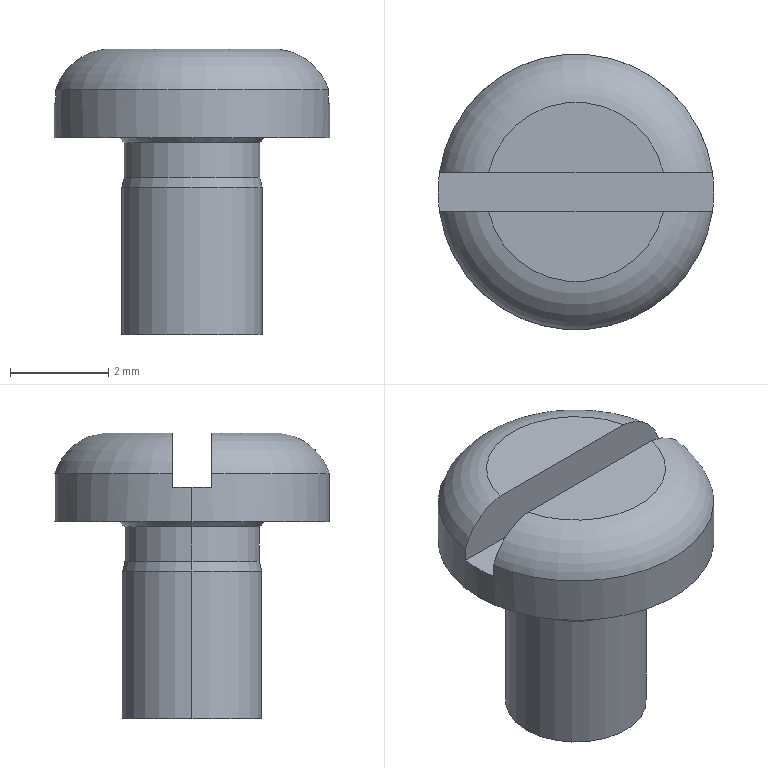Part | SolidWorks | features ICE 3, Revolution 2, Extrusion 1, RevCut 1 | 1 solid | 19 faces | box 5.6 x 5.6 x 5.8 mm | volume 61.126 mm3 | plane 7 | cylinder 6 | torus 4 | cone 2 | commonest cylinder face diameters 2.75 x2 2.85 x2 5.6 x2
STEP:
#1=CARTESIAN_POINT('',(-1.425,0.,-4.));
#2=VERTEX_POINT('',#1);
#3=CARTESIAN_POINT('',(1.425,0.,-4.));
#4=VERTEX_POINT('',#3);
#5=CARTESIAN_POINT('',(0.,0.,-4.));
#6=DIRECTION('',(0.,0.,-1.));
#7=DIRECTION('',(-1.,0.,0.));
#8=AXIS2_PLACEMENT_3D('',#5,#6,#7);
#9=CIRCLE('',#8,1.425);
#10=EDGE_CURVE('',#2,#4,#9,.T.);
#11=ORIENTED_EDGE('',*,*,#10,.F.);
#12=CARTESIAN_POINT('',(-1.425,0.,-1.));
#13=VERTEX_POINT('',#12);
#14=CARTESIAN_POINT('',(-1.425,0.,-4.));
#15=DIRECTION('',(0.,0.,1.));
#16=VECTOR('',#15,1000.);
#17=LINE('',#14,#16);
#18=EDGE_CURVE('',#2,#13,#17,.T.);
#19=ORIENTED_EDGE('',*,*,#18,.T.);
#20=CARTESIAN_POINT('',(1.425,0.,-1.));
#21=VERTEX_POINT('',#20);
#22=CARTESIAN_POINT('',(0.,0.,-1.));
#23=DIRECTION('',(0.,0.,-1.));
#24=DIRECTION('',(-1.,0.,0.));
#25=AXIS2_PLACEMENT_3D('',#22,#23,#24);
#26=CIRCLE('',#25,1.425);
#27=EDGE_CURVE('',#13,#21,#26,.T.);
#28=ORIENTED_EDGE('',*,*,#27,.T.);
#29=CARTESIAN_POINT('',(1.425,0.,-4.));
#30=DIRECTION('',(0.,0.,1.));
#31=VECTOR('',#30,1000.);
#32=LINE('',#29,#31);
#33=EDGE_CURVE('',#4,#21,#32,.T.);
#34=ORIENTED_EDGE('',*,*,#33,.F.);
#35=EDGE_LOOP('',(#11,#19,#28,#34));
#36=FACE_OUTER_BOUND('',#35,.T.);
#37=CARTESIAN_POINT('',(0.,0.,-4.));
#38=DIRECTION('',(0.,0.,1.));
#39=DIRECTION('',(1.,0.,0.));
#40=AXIS2_PLACEMENT_3D('',#37,#38,#39);
#41=CYLINDRICAL_SURFACE('',#40,1.425);
#42=ADVANCED_FACE('',(#36),#41,.T.);
#43=CARTESIAN_POINT('',(-1.375,0.,-0.8));
#44=VERTEX_POINT('',#43);
#45=CARTESIAN_POINT('',(1.375,0.,-0.8));
#46=VERTEX_POINT('',#45);
#47=CARTESIAN_POINT('',(0.,0.,-0.8));
#48=DIRECTION('',(0.,0.,-1.));
#49=DIRECTION('',(-1.,0.,0.));
#50=AXIS2_PLACEMENT_3D('',#47,#48,#49);
#51=CIRCLE('',#50,1.375);
#52=EDGE_CURVE('',#44,#46,#51,.T.);
#53=ORIENTED_EDGE('',*,*,#52,.T.);
#54=CARTESIAN_POINT('',(1.375,0.,-0.8));
#55=DIRECTION('',(0.2425,0.,-0.9701));
#56=VECTOR('',#55,1000.);
#57=LINE('',#54,#56);
#58=EDGE_CURVE('',#46,#21,#57,.T.);
#59=ORIENTED_EDGE('',*,*,#58,.T.);
#60=ORIENTED_EDGE('',*,*,#27,.F.);
#61=CARTESIAN_POINT('',(-1.375,0.,-0.8));
#62=DIRECTION('',(-0.2425,0.,-0.9701));
#63=VECTOR('',#62,1000.);
#64=LINE('',#61,#63);
#65=EDGE_CURVE('',#44,#13,#64,.T.);
#66=ORIENTED_EDGE('',*,*,#65,.F.);
#67=EDGE_LOOP('',(#53,#59,#60,#66));
#68=FACE_OUTER_BOUND('',#67,.T.);
#69=CARTESIAN_POINT('',(0.,0.,-0.8));
#70=DIRECTION('',(0.,0.,-1.));
#71=DIRECTION('',(-1.,0.,0.));
#72=AXIS2_PLACEMENT_3D('',#69,#70,#71);
#73=CONICAL_SURFACE('',#72,1.375,0.245);
#74=ADVANCED_FACE('',(#68),#73,.T.);
#75=ORIENTED_EDGE('',*,*,#52,.F.);
#76=CARTESIAN_POINT('',(-1.375,0.,-0.1));
#77=VERTEX_POINT('',#76);
#78=CARTESIAN_POINT('',(-1.375,0.,-0.8));
#79=DIRECTION('',(0.,0.,1.));
#80=VECTOR('',#79,1000.);
#81=LINE('',#78,#80);
#82=EDGE_CURVE('',#44,#77,#81,.T.);
#83=ORIENTED_EDGE('',*,*,#82,.T.);
#84=CARTESIAN_POINT('',(1.375,0.,-0.1));
#85=VERTEX_POINT('',#84);
#86=CARTESIAN_POINT('',(0.,0.,-0.1));
#87=DIRECTION('',(0.,0.,-1.));
#88=DIRECTION('',(-1.,0.,0.));
#89=AXIS2_PLACEMENT_3D('',#86,#87,#88);
#90=CIRCLE('',#89,1.375);
#91=EDGE_CURVE('',#77,#85,#90,.T.);
#92=ORIENTED_EDGE('',*,*,#91,.T.);
#93=CARTESIAN_POINT('',(1.375,0.,-0.8));
#94=DIRECTION('',(0.,0.,1.));
#95=VECTOR('',#94,1000.);
#96=LINE('',#93,#95);
#97=EDGE_CURVE('',#46,#85,#96,.T.);
#98=ORIENTED_EDGE('',*,*,#97,.F.);
#99=EDGE_LOOP('',(#75,#83,#92,#98));
#100=FACE_OUTER_BOUND('',#99,.T.);
#101=CARTESIAN_POINT('',(0.,0.,-0.8));
#102=DIRECTION('',(0.,0.,1.));
#103=DIRECTION('',(1.,0.,0.));
#104=AXIS2_PLACEMENT_3D('',#101,#102,#103);
#105=CYLINDRICAL_SURFACE('',#104,1.375);
#106=ADVANCED_FACE('',(#100),#105,.T.);
#107=CARTESIAN_POINT('',(-1.475,0.,0.));
#108=VERTEX_POINT('',#107);
#109=CARTESIAN_POINT('',(1.475,0.,0.));
#110=VERTEX_POINT('',#109);
#111=CARTESIAN_POINT('',(0.,0.,0.));
#112=DIRECTION('',(0.,0.,1.));
#113=DIRECTION('',(1.,0.,0.));
#114=AXIS2_PLACEMENT_3D('',#111,#112,#113);
#115=CIRCLE('',#114,1.475);
#116=EDGE_CURVE('',#108,#110,#115,.T.);
#117=ORIENTED_EDGE('',*,*,#116,.F.);
#118=CARTESIAN_POINT('',(-2.048,0.,-0.673));
#119=DIRECTION('',(0.,1.,0.));
#120=DIRECTION('',(-1.,0.,0.));
#121=AXIS2_PLACEMENT_3D('',#118,#119,#120);
#122=CIRCLE('',#121,0.8839);
#123=EDGE_CURVE('',#108,#77,#122,.T.);
#124=ORIENTED_EDGE('',*,*,#123,.T.);
#125=CARTESIAN_POINT('',(0.,0.,-0.1));
#126=DIRECTION('',(0.,0.,-1.));
#127=DIRECTION('',(-1.,0.,0.));
#128=AXIS2_PLACEMENT_3D('',#125,#126,#127);
#129=CIRCLE('',#128,1.375);
#130=EDGE_CURVE('',#85,#77,#129,.T.);
#131=ORIENTED_EDGE('',*,*,#130,.F.);
#132=CARTESIAN_POINT('',(2.048,0.,-0.673));
#133=DIRECTION('',(0.,-1.,0.));
#134=DIRECTION('',(0.,0.,-1.));
#135=AXIS2_PLACEMENT_3D('',#132,#133,#134);
#136=CIRCLE('',#135,0.8839);
#137=EDGE_CURVE('',#110,#85,#136,.T.);
#138=ORIENTED_EDGE('',*,*,#137,.F.);
#139=EDGE_LOOP('',(#117,#124,#131,#138));
#140=FACE_OUTER_BOUND('',#139,.T.);
#141=CARTESIAN_POINT('',(0.,0.,-0.673));
#142=DIRECTION('',(0.,0.,1.));
#143=DIRECTION('',(1.,0.,0.));
#144=AXIS2_PLACEMENT_3D('',#141,#142,#143);
#145=TOROIDAL_SURFACE('',#144,2.048,0.8839);
#146=ADVANCED_FACE('',(#140),#145,.F.);
#147=CARTESIAN_POINT('',(2.771,0.4,0.7));
#148=VERTEX_POINT('',#147);
#149=CARTESIAN_POINT('',(2.8,0.,0.7));
#150=VERTEX_POINT('',#149);
#151=CARTESIAN_POINT('',(0.,0.,0.7));
#152=DIRECTION('',(0.,0.,-1.));
#153=DIRECTION('',(-1.,0.,0.));
#154=AXIS2_PLACEMENT_3D('',#151,#152,#153);
#155=CIRCLE('',#154,2.8);
#156=EDGE_CURVE('',#148,#150,#155,.T.);
#157=ORIENTED_EDGE('',*,*,#156,.T.);
#158=CARTESIAN_POINT('',(2.8,0.,0.));
#159=VERTEX_POINT('',#158);
#160=CARTESIAN_POINT('',(2.8,0.,1.8));
#161=DIRECTION('',(0.,0.,-1.));
#162=VECTOR('',#161,1000.);
#163=LINE('',#160,#162);
#164=EDGE_CURVE('',#150,#159,#163,.T.);
#165=ORIENTED_EDGE('',*,*,#164,.T.);
#166=CARTESIAN_POINT('',(-2.8,0.,0.));
#167=VERTEX_POINT('',#166);
#168=CARTESIAN_POINT('',(0.,0.,0.));
#169=DIRECTION('',(0.,0.,1.));
#170=DIRECTION('',(1.,0.,0.));
#171=AXIS2_PLACEMENT_3D('',#168,#169,#170);
#172=CIRCLE('',#171,2.8);
#173=EDGE_CURVE('',#159,#167,#172,.T.);
#174=ORIENTED_EDGE('',*,*,#173,.T.);
#175=CARTESIAN_POINT('',(-2.8,0.,0.7));
#176=VERTEX_POINT('',#175);
#177=CARTESIAN_POINT('',(-2.8,0.,1.8));
#178=DIRECTION('',(0.,0.,-1.));
#179=VECTOR('',#178,1000.);
#180=LINE('',#177,#179);
#181=EDGE_CURVE('',#176,#167,#180,.T.);
#182=ORIENTED_EDGE('',*,*,#181,.F.);
#183=CARTESIAN_POINT('',(-2.771,0.4,0.7));
#184=VERTEX_POINT('',#183);
#185=CARTESIAN_POINT('',(0.,0.,0.7));
#186=DIRECTION('',(0.,0.,-1.));
#187=DIRECTION('',(-1.,0.,0.));
#188=AXIS2_PLACEMENT_3D('',#185,#186,#187);
#189=CIRCLE('',#188,2.8);
#190=EDGE_CURVE('',#176,#184,#189,.T.);
#191=ORIENTED_EDGE('',*,*,#190,.T.);
#192=CARTESIAN_POINT('',(-2.771,0.4,0.98));
#193=VERTEX_POINT('',#192);
#194=CARTESIAN_POINT('',(-2.771,0.4,1.8));
#195=DIRECTION('',(0.,0.,1.));
#196=VECTOR('',#195,1000.);
#197=LINE('',#194,#196);
#198=EDGE_CURVE('',#184,#193,#197,.T.);
#199=ORIENTED_EDGE('',*,*,#198,.T.);
#200=CARTESIAN_POINT('',(2.771,0.4,0.98));
#201=VERTEX_POINT('',#200);
#202=CARTESIAN_POINT('',(0.,0.,0.98));
#203=DIRECTION('',(0.,0.,-1.));
#204=DIRECTION('',(-1.,0.,0.));
#205=AXIS2_PLACEMENT_3D('',#202,#203,#204);
#206=CIRCLE('',#205,2.8);
#207=EDGE_CURVE('',#193,#201,#206,.T.);
#208=ORIENTED_EDGE('',*,*,#207,.T.);
#209=CARTESIAN_POINT('',(2.771,0.4,1.8));
#210=DIRECTION('',(0.,0.,-1.));
#211=VECTOR('',#210,1000.);
#212=LINE('',#209,#211);
#213=EDGE_CURVE('',#201,#148,#212,.T.);
#214=ORIENTED_EDGE('',*,*,#213,.T.);
#215=EDGE_LOOP('',(#157,#165,#174,#182,#191,#199,#208,#214));
#216=FACE_OUTER_BOUND('',#215,.T.);
#217=CARTESIAN_POINT('',(0.,0.,1.8));
#218=DIRECTION('',(0.,0.,-1.));
#219=DIRECTION('',(-1.,0.,0.));
#220=AXIS2_PLACEMENT_3D('',#217,#218,#219);
#221=CYLINDRICAL_SURFACE('',#220,2.8);
#222=ADVANCED_FACE('',(#216),#221,.T.);
#223=CARTESIAN_POINT('',(-2.771,-0.4,0.98));
#224=VERTEX_POINT('',#223);
#225=CARTESIAN_POINT('',(-1.775,-0.4,1.8));
#226=VERTEX_POINT('',#225);
#227=CARTESIAN_POINT('',(-2.771,-0.4,0.98));
#228=CARTESIAN_POINT('',(-2.737,-0.4,1.088));
#229=CARTESIAN_POINT('',(-2.687,-0.4,1.191));
#230=CARTESIAN_POINT('',(-2.559,-0.4,1.38));
#231=CARTESIAN_POINT('',(-2.481,-0.4,1.465));
#232=CARTESIAN_POINT('',(-2.306,-0.4,1.608));
#233=CARTESIAN_POINT('',(-2.207,-0.4,1.667));
#234=CARTESIAN_POINT('',(-1.998,-0.4,1.756));
#235=CARTESIAN_POINT('',(-1.889,-0.4,1.786));
#236=CARTESIAN_POINT('',(-1.775,-0.4,1.8));
#237=B_SPLINE_CURVE_WITH_KNOTS('',3,(#227,#228,#229,#230,#231,#232,#233,#234,#235,#236),.UNSPECIFIED.,.F.,.F.,(4,2,2,2,4),(0.00711,0.007449,0.007788,0.008126,0.008465),.UNSPECIFIED.);
#238=EDGE_CURVE('',#224,#226,#237,.T.);
#239=ORIENTED_EDGE('',*,*,#238,.F.);
#240=CARTESIAN_POINT('',(2.771,-0.4,0.98));
#241=VERTEX_POINT('',#240);
#242=CARTESIAN_POINT('',(0.,0.,0.98));
#243=DIRECTION('',(0.,0.,-1.));
#244=DIRECTION('',(-1.,0.,0.));
#245=AXIS2_PLACEMENT_3D('',#242,#243,#244);
#246=CIRCLE('',#245,2.8);
#247=EDGE_CURVE('',#241,#224,#246,.T.);
#248=ORIENTED_EDGE('',*,*,#247,.F.);
#249=CARTESIAN_POINT('',(1.775,-0.4,1.8));
#250=VERTEX_POINT('',#249);
#251=CARTESIAN_POINT('',(1.775,-0.4,1.8));
#252=CARTESIAN_POINT('',(2.,-0.4,1.772));
#253=CARTESIAN_POINT('',(2.219,-0.4,1.679));
#254=CARTESIAN_POINT('',(2.482,-0.4,1.464));
#255=CARTESIAN_POINT('',(2.559,-0.4,1.379));
#256=CARTESIAN_POINT('',(2.687,-0.4,1.191));
#257=CARTESIAN_POINT('',(2.737,-0.4,1.089));
#258=CARTESIAN_POINT('',(2.771,-0.4,0.98));
#259=B_SPLINE_CURVE_WITH_KNOTS('',3,(#251,#252,#253,#254,#255,#256,#257,#258),.UNSPECIFIED.,.F.,.F.,(4,2,2,4),(0.001738,0.002418,0.002758,0.003097),.UNSPECIFIED.);
#260=EDGE_CURVE('',#250,#241,#259,.T.);
#261=ORIENTED_EDGE('',*,*,#260,.F.);
#262=CARTESIAN_POINT('',(0.,0.,1.8));
#263=DIRECTION('',(0.,0.,-1.));
#264=DIRECTION('',(-1.,0.,0.));
#265=AXIS2_PLACEMENT_3D('',#262,#263,#264);
#266=CIRCLE('',#265,1.82);
#267=EDGE_CURVE('',#250,#226,#266,.T.);
#268=ORIENTED_EDGE('',*,*,#267,.T.);
#269=EDGE_LOOP('',(#239,#248,#261,#268));
#270=FACE_OUTER_BOUND('',#269,.T.);
#271=CARTESIAN_POINT('',(0.,0.,0.624));
#272=DIRECTION('',(0.,0.,-1.));
#273=DIRECTION('',(-1.,0.,0.));
#274=AXIS2_PLACEMENT_3D('',#271,#272,#273);
#275=TOROIDAL_SURFACE('',#274,1.669,1.186);
#276=ADVANCED_FACE('',(#270),#275,.T.);
#277=CARTESIAN_POINT('',(0.,-0.4,1.8));
#278=DIRECTION('',(1.,0.,0.));
#279=VECTOR('',#278,1000.);
#280=LINE('',#277,#279);
#281=EDGE_CURVE('',#226,#250,#280,.T.);
#282=ORIENTED_EDGE('',*,*,#281,.F.);
#283=ORIENTED_EDGE('',*,*,#267,.F.);
#284=EDGE_LOOP('',(#282,#283));
#285=FACE_OUTER_BOUND('',#284,.T.);
#286=CARTESIAN_POINT('',(0.,0.,1.8));
#287=DIRECTION('',(0.,0.,1.));
#288=DIRECTION('',(1.,0.,0.));
#289=AXIS2_PLACEMENT_3D('',#286,#287,#288);
#290=PLANE('',#289);
#291=ADVANCED_FACE('',(#285),#290,.T.);
#292=ORIENTED_EDGE('',*,*,#164,.F.);
#293=CARTESIAN_POINT('',(2.771,-0.4,0.7));
#294=VERTEX_POINT('',#293);
#295=CARTESIAN_POINT('',(0.,0.,0.7));
#296=DIRECTION('',(0.,0.,-1.));
#297=DIRECTION('',(-1.,0.,0.));
#298=AXIS2_PLACEMENT_3D('',#295,#296,#297);
#299=CIRCLE('',#298,2.8);
#300=EDGE_CURVE('',#150,#294,#299,.T.);
#301=ORIENTED_EDGE('',*,*,#300,.T.);
#302=CARTESIAN_POINT('',(2.771,-0.4,1.8));
#303=DIRECTION('',(0.,0.,1.));
#304=VECTOR('',#303,1000.);
#305=LINE('',#302,#304);
#306=EDGE_CURVE('',#294,#241,#305,.T.);
#307=ORIENTED_EDGE('',*,*,#306,.T.);
#308=ORIENTED_EDGE('',*,*,#247,.T.);
#309=CARTESIAN_POINT('',(-2.771,-0.4,0.7));
#310=VERTEX_POINT('',#309);
#311=CARTESIAN_POINT('',(-2.771,-0.4,1.8));
#312=DIRECTION('',(0.,0.,-1.));
#313=VECTOR('',#312,1000.);
#314=LINE('',#311,#313);
#315=EDGE_CURVE('',#224,#310,#314,.T.);
#316=ORIENTED_EDGE('',*,*,#315,.T.);
#317=CARTESIAN_POINT('',(0.,0.,0.7));
#318=DIRECTION('',(0.,0.,-1.));
#319=DIRECTION('',(-1.,0.,0.));
#320=AXIS2_PLACEMENT_3D('',#317,#318,#319);
#321=CIRCLE('',#320,2.8);
#322=EDGE_CURVE('',#310,#176,#321,.T.);
#323=ORIENTED_EDGE('',*,*,#322,.T.);
#324=ORIENTED_EDGE('',*,*,#181,.T.);
#325=CARTESIAN_POINT('',(0.,0.,0.));
#326=DIRECTION('',(0.,0.,1.));
#327=DIRECTION('',(1.,0.,0.));
#328=AXIS2_PLACEMENT_3D('',#325,#326,#327);
#329=CIRCLE('',#328,2.8);
#330=EDGE_CURVE('',#167,#159,#329,.T.);
#331=ORIENTED_EDGE('',*,*,#330,.T.);
#332=EDGE_LOOP('',(#292,#301,#307,#308,#316,#323,#324,#331));
#333=FACE_OUTER_BOUND('',#332,.T.);
#334=CARTESIAN_POINT('',(0.,0.,1.8));
#335=DIRECTION('',(0.,0.,-1.));
#336=DIRECTION('',(-1.,0.,0.));
#337=AXIS2_PLACEMENT_3D('',#334,#335,#336);
#338=CYLINDRICAL_SURFACE('',#337,2.8);
#339=ADVANCED_FACE('',(#333),#338,.T.);
#340=CARTESIAN_POINT('',(0.,0.,0.));
#341=DIRECTION('',(0.,0.,1.));
#342=DIRECTION('',(1.,0.,0.));
#343=AXIS2_PLACEMENT_3D('',#340,#341,#342);
#344=CIRCLE('',#343,1.475);
#345=EDGE_CURVE('',#110,#108,#344,.T.);
#346=ORIENTED_EDGE('',*,*,#345,.T.);
#347=ORIENTED_EDGE('',*,*,#116,.T.);
#348=EDGE_LOOP('',(#346,#347));
#349=FACE_BOUND('',#348,.T.);
#350=ORIENTED_EDGE('',*,*,#330,.F.);
#351=ORIENTED_EDGE('',*,*,#173,.F.);
#352=EDGE_LOOP('',(#350,#351));
#353=FACE_OUTER_BOUND('',#352,.T.);
#354=CARTESIAN_POINT('',(0.,0.,0.));
#355=DIRECTION('',(0.,0.,1.));
#356=DIRECTION('',(1.,0.,0.));
#357=AXIS2_PLACEMENT_3D('',#354,#355,#356);
#358=PLANE('',#357);
#359=ADVANCED_FACE('',(#349,#353),#358,.F.);
#360=ORIENTED_EDGE('',*,*,#123,.F.);
#361=ORIENTED_EDGE('',*,*,#345,.F.);
#362=ORIENTED_EDGE('',*,*,#137,.T.);
#363=ORIENTED_EDGE('',*,*,#91,.F.);
#364=EDGE_LOOP('',(#360,#361,#362,#363));
#365=FACE_OUTER_BOUND('',#364,.T.);
#366=CARTESIAN_POINT('',(0.,0.,-0.673));
#367=DIRECTION('',(0.,0.,1.));
#368=DIRECTION('',(1.,0.,0.));
#369=AXIS2_PLACEMENT_3D('',#366,#367,#368);
#370=TOROIDAL_SURFACE('',#369,2.048,0.8839);
#371=ADVANCED_FACE('',(#365),#370,.F.);
#372=ORIENTED_EDGE('',*,*,#82,.F.);
#373=CARTESIAN_POINT('',(0.,0.,-0.8));
#374=DIRECTION('',(0.,0.,-1.));
#375=DIRECTION('',(-1.,0.,0.));
#376=AXIS2_PLACEMENT_3D('',#373,#374,#375);
#377=CIRCLE('',#376,1.375);
#378=EDGE_CURVE('',#46,#44,#377,.T.);
#379=ORIENTED_EDGE('',*,*,#378,.F.);
#380=ORIENTED_EDGE('',*,*,#97,.T.);
#381=ORIENTED_EDGE('',*,*,#130,.T.);
#382=EDGE_LOOP('',(#372,#379,#380,#381));
#383=FACE_OUTER_BOUND('',#382,.T.);
#384=CARTESIAN_POINT('',(0.,0.,-0.8));
#385=DIRECTION('',(0.,0.,1.));
#386=DIRECTION('',(1.,0.,0.));
#387=AXIS2_PLACEMENT_3D('',#384,#385,#386);
#388=CYLINDRICAL_SURFACE('',#387,1.375);
#389=ADVANCED_FACE('',(#383),#388,.T.);
#390=ORIENTED_EDGE('',*,*,#58,.F.);
#391=ORIENTED_EDGE('',*,*,#378,.T.);
#392=ORIENTED_EDGE('',*,*,#65,.T.);
#393=CARTESIAN_POINT('',(0.,0.,-1.));
#394=DIRECTION('',(0.,0.,-1.));
#395=DIRECTION('',(-1.,0.,0.));
#396=AXIS2_PLACEMENT_3D('',#393,#394,#395);
#397=CIRCLE('',#396,1.425);
#398=EDGE_CURVE('',#21,#13,#397,.T.);
#399=ORIENTED_EDGE('',*,*,#398,.F.);
#400=EDGE_LOOP('',(#390,#391,#392,#399));
#401=FACE_OUTER_BOUND('',#400,.T.);
#402=CARTESIAN_POINT('',(0.,0.,-0.8));
#403=DIRECTION('',(0.,0.,-1.));
#404=DIRECTION('',(-1.,0.,0.));
#405=AXIS2_PLACEMENT_3D('',#402,#403,#404);
#406=CONICAL_SURFACE('',#405,1.375,0.245);
#407=ADVANCED_FACE('',(#401),#406,.T.);
#408=ORIENTED_EDGE('',*,*,#18,.F.);
#409=CARTESIAN_POINT('',(0.,0.,-4.));
#410=DIRECTION('',(0.,0.,-1.));
#411=DIRECTION('',(-1.,0.,0.));
#412=AXIS2_PLACEMENT_3D('',#409,#410,#411);
#413=CIRCLE('',#412,1.425);
#414=EDGE_CURVE('',#4,#2,#413,.T.);
#415=ORIENTED_EDGE('',*,*,#414,.F.);
#416=ORIENTED_EDGE('',*,*,#33,.T.);
#417=ORIENTED_EDGE('',*,*,#398,.T.);
#418=EDGE_LOOP('',(#408,#415,#416,#417));
#419=FACE_OUTER_BOUND('',#418,.T.);
#420=CARTESIAN_POINT('',(0.,0.,-4.));
#421=DIRECTION('',(0.,0.,1.));
#422=DIRECTION('',(1.,0.,0.));
#423=AXIS2_PLACEMENT_3D('',#420,#421,#422);
#424=CYLINDRICAL_SURFACE('',#423,1.425);
#425=ADVANCED_FACE('',(#419),#424,.T.);
#426=ORIENTED_EDGE('',*,*,#414,.T.);
#427=ORIENTED_EDGE('',*,*,#10,.T.);
#428=EDGE_LOOP('',(#426,#427));
#429=FACE_OUTER_BOUND('',#428,.T.);
#430=CARTESIAN_POINT('',(0.,0.,-4.));
#431=DIRECTION('',(0.,0.,-1.));
#432=DIRECTION('',(-1.,0.,0.));
#433=AXIS2_PLACEMENT_3D('',#430,#431,#432);
#434=PLANE('',#433);
#435=ADVANCED_FACE('',(#429),#434,.T.);
#436=CARTESIAN_POINT('',(-1.775,0.4,1.8));
#437=VERTEX_POINT('',#436);
#438=CARTESIAN_POINT('',(-1.775,0.4,1.8));
#439=CARTESIAN_POINT('',(-1.889,0.4,1.786));
#440=CARTESIAN_POINT('',(-1.998,0.4,1.757));
#441=CARTESIAN_POINT('',(-2.207,0.4,1.667));
#442=CARTESIAN_POINT('',(-2.305,0.4,1.608));
#443=CARTESIAN_POINT('',(-2.568,0.4,1.393));
#444=CARTESIAN_POINT('',(-2.703,0.4,1.196));
#445=CARTESIAN_POINT('',(-2.771,0.4,0.98));
#446=B_SPLINE_CURVE_WITH_KNOTS('',3,(#438,#439,#440,#441,#442,#443,#444,#445),.UNSPECIFIED.,.F.,.F.,(4,2,2,4),(0.006821,0.00716,0.0075,0.008179),.UNSPECIFIED.);
#447=EDGE_CURVE('',#437,#193,#446,.T.);
#448=ORIENTED_EDGE('',*,*,#447,.F.);
#449=CARTESIAN_POINT('',(1.775,0.4,1.8));
#450=VERTEX_POINT('',#449);
#451=CARTESIAN_POINT('',(0.,0.,1.8));
#452=DIRECTION('',(0.,0.,-1.));
#453=DIRECTION('',(-1.,0.,0.));
#454=AXIS2_PLACEMENT_3D('',#451,#452,#453);
#455=CIRCLE('',#454,1.82);
#456=EDGE_CURVE('',#437,#450,#455,.T.);
#457=ORIENTED_EDGE('',*,*,#456,.T.);
#458=CARTESIAN_POINT('',(2.771,0.4,0.98));
#459=CARTESIAN_POINT('',(2.702,0.4,1.197));
#460=CARTESIAN_POINT('',(2.57,0.4,1.391));
#461=CARTESIAN_POINT('',(2.218,0.4,1.68));
#462=CARTESIAN_POINT('',(2.,0.4,1.772));
#463=CARTESIAN_POINT('',(1.775,0.4,1.8));
#464=B_SPLINE_CURVE_WITH_KNOTS('',3,(#458,#459,#460,#461,#462,#463),.UNSPECIFIED.,.F.,.F.,(4,2,4),(0.004547,0.005224,0.005901),.UNSPECIFIED.);
#465=EDGE_CURVE('',#201,#450,#464,.T.);
#466=ORIENTED_EDGE('',*,*,#465,.F.);
#467=ORIENTED_EDGE('',*,*,#207,.F.);
#468=EDGE_LOOP('',(#448,#457,#466,#467));
#469=FACE_OUTER_BOUND('',#468,.T.);
#470=CARTESIAN_POINT('',(0.,0.,0.624));
#471=DIRECTION('',(0.,0.,-1.));
#472=DIRECTION('',(-1.,0.,0.));
#473=AXIS2_PLACEMENT_3D('',#470,#471,#472);
#474=TOROIDAL_SURFACE('',#473,1.669,1.186);
#475=ADVANCED_FACE('',(#469),#474,.T.);
#476=CARTESIAN_POINT('',(0.,0.4,1.8));
#477=DIRECTION('',(-1.,0.,0.));
#478=VECTOR('',#477,1000.);
#479=LINE('',#476,#478);
#480=EDGE_CURVE('',#450,#437,#479,.T.);
#481=ORIENTED_EDGE('',*,*,#480,.F.);
#482=ORIENTED_EDGE('',*,*,#456,.F.);
#483=EDGE_LOOP('',(#481,#482));
#484=FACE_OUTER_BOUND('',#483,.T.);
#485=CARTESIAN_POINT('',(0.,0.,1.8));
#486=DIRECTION('',(0.,0.,1.));
#487=DIRECTION('',(1.,0.,0.));
#488=AXIS2_PLACEMENT_3D('',#485,#486,#487);
#489=PLANE('',#488);
#490=ADVANCED_FACE('',(#484),#489,.T.);
#491=CARTESIAN_POINT('',(2.8,0.4,0.7));
#492=DIRECTION('',(-1.,0.,0.));
#493=VECTOR('',#492,1000.);
#494=LINE('',#491,#493);
#495=EDGE_CURVE('',#148,#184,#494,.T.);
#496=ORIENTED_EDGE('',*,*,#495,.T.);
#497=ORIENTED_EDGE('',*,*,#190,.F.);
#498=ORIENTED_EDGE('',*,*,#322,.F.);
#499=CARTESIAN_POINT('',(2.8,-0.4,0.7));
#500=DIRECTION('',(-1.,0.,0.));
#501=VECTOR('',#500,1000.);
#502=LINE('',#499,#501);
#503=EDGE_CURVE('',#294,#310,#502,.T.);
#504=ORIENTED_EDGE('',*,*,#503,.F.);
#505=ORIENTED_EDGE('',*,*,#300,.F.);
#506=ORIENTED_EDGE('',*,*,#156,.F.);
#507=EDGE_LOOP('',(#496,#497,#498,#504,#505,#506));
#508=FACE_OUTER_BOUND('',#507,.T.);
#509=CARTESIAN_POINT('',(2.8,-0.4,0.7));
#510=DIRECTION('',(0.,0.,-1.));
#511=DIRECTION('',(-1.,0.,0.));
#512=AXIS2_PLACEMENT_3D('',#509,#510,#511);
#513=PLANE('',#512);
#514=ADVANCED_FACE('',(#508),#513,.F.);
#515=ORIENTED_EDGE('',*,*,#238,.T.);
#516=ORIENTED_EDGE('',*,*,#281,.T.);
#517=ORIENTED_EDGE('',*,*,#260,.T.);
#518=ORIENTED_EDGE('',*,*,#306,.F.);
#519=ORIENTED_EDGE('',*,*,#503,.T.);
#520=ORIENTED_EDGE('',*,*,#315,.F.);
#521=EDGE_LOOP('',(#515,#516,#517,#518,#519,#520));
#522=FACE_OUTER_BOUND('',#521,.T.);
#523=CARTESIAN_POINT('',(2.8,-0.4,0.7));
#524=DIRECTION('',(0.,-1.,0.));
#525=DIRECTION('',(0.,0.,-1.));
#526=AXIS2_PLACEMENT_3D('',#523,#524,#525);
#527=PLANE('',#526);
#528=ADVANCED_FACE('',(#522),#527,.F.);
#529=ORIENTED_EDGE('',*,*,#465,.T.);
#530=ORIENTED_EDGE('',*,*,#480,.T.);
#531=ORIENTED_EDGE('',*,*,#447,.T.);
#532=ORIENTED_EDGE('',*,*,#198,.F.);
#533=ORIENTED_EDGE('',*,*,#495,.F.);
#534=ORIENTED_EDGE('',*,*,#213,.F.);
#535=EDGE_LOOP('',(#529,#530,#531,#532,#533,#534));
#536=FACE_OUTER_BOUND('',#535,.T.);
#537=CARTESIAN_POINT('',(2.8,0.4,2.068));
#538=DIRECTION('',(0.,1.,0.));
#539=DIRECTION('',(0.,0.,1.));
#540=AXIS2_PLACEMENT_3D('',#537,#538,#539);
#541=PLANE('',#540);
#542=ADVANCED_FACE('',(#536),#541,.F.);
#543=CLOSED_SHELL('',(#42,#74,#106,#146,#222,#276,#291,#339,#359,#371,#389,#407,#425,#435,#475,#490,#514,#528,#542));
#544=MANIFOLD_SOLID_BREP('',#543);
#545=CARTESIAN_POINT('',(0.,0.,0.));
#546=DIRECTION('',(0.,0.,1.));
#547=DIRECTION('',(1.,0.,0.));
#548=AXIS2_PLACEMENT_3D('',#545,#546,#547);
#549=(LENGTH_UNIT()NAMED_UNIT(*)SI_UNIT(.MILLI.,.METRE.));
#550=UNCERTAINTY_MEASURE_WITH_UNIT(LENGTH_MEASURE(0.00001),#549,'','');
#551=(NAMED_UNIT(*)PLANE_ANGLE_UNIT()SI_UNIT($,.RADIAN.));
#552=(NAMED_UNIT(*)SI_UNIT($,.STERADIAN.)SOLID_ANGLE_UNIT());
#553=(GEOMETRIC_REPRESENTATION_CONTEXT(3)GLOBAL_UNCERTAINTY_ASSIGNED_CONTEXT((#550))GLOBAL_UNIT_ASSIGNED_CONTEXT((#549,#551,#552))REPRESENTATION_CONTEXT('',''));
#554=ADVANCED_BREP_SHAPE_REPRESENTATION('',(#544,#548),#553);